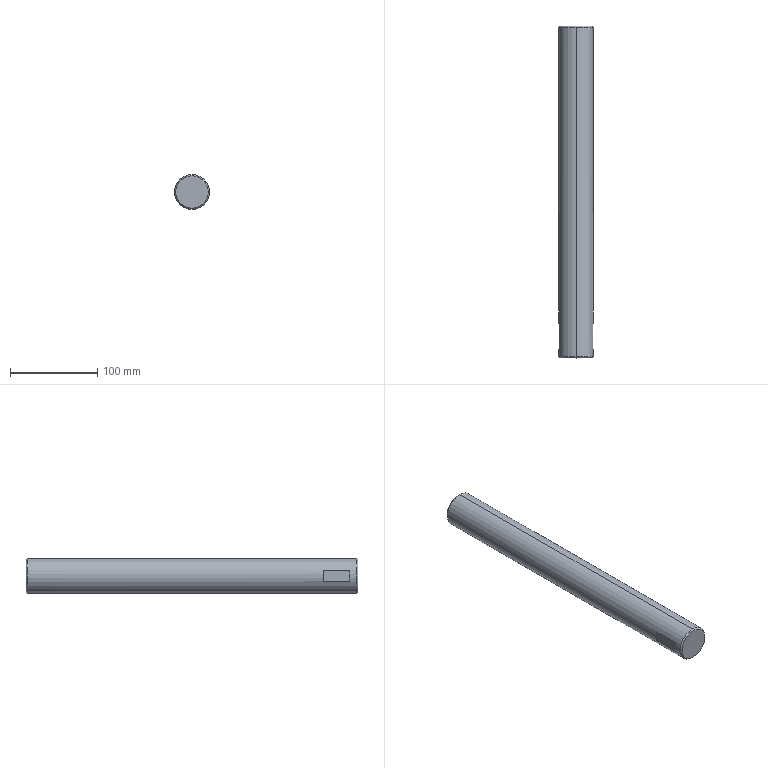Part | SolidWorks | features Chamfer 1, HoleWzd 1, ICE 1, Revolution 1 | 1 solid | 18 faces | box 40 x 380 x 40 mm | volume 474700 mm3 | plane 8 | cone 6 | cylinder 4 | commonest cylinder face diameters 10.2 x2 40 x2
STEP:
#1=CARTESIAN_POINT('',(-88.746,301.337,-5.1));
#2=VERTEX_POINT('',#1);
#3=CARTESIAN_POINT('',(-88.746,301.337,5.1));
#4=VERTEX_POINT('',#3);
#5=CARTESIAN_POINT('',(-88.746,301.337,0.));
#6=DIRECTION('',(0.,1.,0.));
#7=DIRECTION('',(0.,0.,1.));
#8=AXIS2_PLACEMENT_3D('',#5,#6,#7);
#9=CIRCLE('',#8,5.1);
#10=EDGE_CURVE('',#2,#4,#9,.T.);
#11=ORIENTED_EDGE('',*,*,#10,.F.);
#12=CARTESIAN_POINT('',(-88.746,325.337,-5.1));
#13=VERTEX_POINT('',#12);
#14=CARTESIAN_POINT('',(-88.746,325.337,-5.1));
#15=DIRECTION('',(0.,1.,0.));
#16=VECTOR('',#15,1000.);
#17=LINE('',#14,#16);
#18=EDGE_CURVE('',#2,#13,#17,.T.);
#19=ORIENTED_EDGE('',*,*,#18,.T.);
#20=CARTESIAN_POINT('',(-88.746,325.337,5.1));
#21=VERTEX_POINT('',#20);
#22=CARTESIAN_POINT('',(-88.746,325.337,0.));
#23=DIRECTION('',(0.,1.,0.));
#24=DIRECTION('',(0.,0.,1.));
#25=AXIS2_PLACEMENT_3D('',#22,#23,#24);
#26=CIRCLE('',#25,5.1);
#27=EDGE_CURVE('',#13,#21,#26,.T.);
#28=ORIENTED_EDGE('',*,*,#27,.T.);
#29=CARTESIAN_POINT('',(-88.746,325.337,5.1));
#30=DIRECTION('',(0.,1.,0.));
#31=VECTOR('',#30,1000.);
#32=LINE('',#29,#31);
#33=EDGE_CURVE('',#4,#21,#32,.T.);
#34=ORIENTED_EDGE('',*,*,#33,.F.);
#35=EDGE_LOOP('',(#11,#19,#28,#34));
#36=FACE_OUTER_BOUND('',#35,.T.);
#37=CARTESIAN_POINT('',(-88.746,325.337,0.));
#38=DIRECTION('',(0.,1.,0.));
#39=DIRECTION('',(0.,0.,1.));
#40=AXIS2_PLACEMENT_3D('',#37,#38,#39);
#41=CYLINDRICAL_SURFACE('',#40,5.1);
#42=ADVANCED_FACE('',(#36),#41,.F.);
#43=CARTESIAN_POINT('',(-88.746,298.273,0.));
#44=VERTEX_POINT('',#43);
#45=CARTESIAN_POINT('',(-88.746,301.337,5.1));
#46=DIRECTION('',(0.,0.515,0.8572));
#47=VECTOR('',#46,1000.);
#48=LINE('',#45,#47);
#49=EDGE_CURVE('',#44,#4,#48,.T.);
#50=ORIENTED_EDGE('',*,*,#49,.F.);
#51=CARTESIAN_POINT('',(-88.746,301.337,-5.1));
#52=DIRECTION('',(0.,0.515,-0.8572));
#53=VECTOR('',#52,1000.);
#54=LINE('',#51,#53);
#55=EDGE_CURVE('',#44,#2,#54,.T.);
#56=ORIENTED_EDGE('',*,*,#55,.T.);
#57=ORIENTED_EDGE('',*,*,#10,.T.);
#58=EDGE_LOOP('',(#50,#56,#57));
#59=FACE_OUTER_BOUND('',#58,.T.);
#60=CARTESIAN_POINT('',(-88.746,301.337,0.));
#61=DIRECTION('',(0.,1.,0.));
#62=DIRECTION('',(0.,0.,1.));
#63=AXIS2_PLACEMENT_3D('',#60,#61,#62);
#64=CONICAL_SURFACE('',#63,5.1,1.03);
#65=ADVANCED_FACE('',(#59),#64,.F.);
#66=CARTESIAN_POINT('',(-88.746,-54.663,-18.5));
#67=VERTEX_POINT('',#66);
#68=CARTESIAN_POINT('',(-88.746,-54.663,18.5));
#69=VERTEX_POINT('',#68);
#70=CARTESIAN_POINT('',(-88.746,-54.663,0.));
#71=DIRECTION('',(0.,-1.,0.));
#72=DIRECTION('',(0.,0.,-1.));
#73=AXIS2_PLACEMENT_3D('',#70,#71,#72);
#74=CIRCLE('',#73,18.5);
#75=EDGE_CURVE('',#67,#69,#74,.T.);
#76=ORIENTED_EDGE('',*,*,#75,.F.);
#77=CARTESIAN_POINT('',(-88.746,-53.163,-20.));
#78=VERTEX_POINT('',#77);
#79=CARTESIAN_POINT('',(-88.746,-53.163,-20.));
#80=DIRECTION('',(0.,0.7071,-0.7071));
#81=VECTOR('',#80,1000.);
#82=LINE('',#79,#81);
#83=EDGE_CURVE('',#67,#78,#82,.T.);
#84=ORIENTED_EDGE('',*,*,#83,.T.);
#85=CARTESIAN_POINT('',(-88.746,-53.163,20.));
#86=VERTEX_POINT('',#85);
#87=CARTESIAN_POINT('',(-88.746,-53.163,0.));
#88=DIRECTION('',(0.,1.,0.));
#89=DIRECTION('',(0.,0.,-1.));
#90=AXIS2_PLACEMENT_3D('',#87,#88,#89);
#91=CIRCLE('',#90,20.);
#92=EDGE_CURVE('',#86,#78,#91,.T.);
#93=ORIENTED_EDGE('',*,*,#92,.F.);
#94=CARTESIAN_POINT('',(-88.746,-53.163,20.));
#95=DIRECTION('',(0.,0.7071,0.7071));
#96=VECTOR('',#95,1000.);
#97=LINE('',#94,#96);
#98=EDGE_CURVE('',#69,#86,#97,.T.);
#99=ORIENTED_EDGE('',*,*,#98,.F.);
#100=EDGE_LOOP('',(#76,#84,#93,#99));
#101=FACE_OUTER_BOUND('',#100,.T.);
#102=CARTESIAN_POINT('',(-88.746,-53.163,0.));
#103=DIRECTION('',(0.,1.,0.));
#104=DIRECTION('',(0.,0.,1.));
#105=AXIS2_PLACEMENT_3D('',#102,#103,#104);
#106=CONICAL_SURFACE('',#105,20.,0.7854);
#107=ADVANCED_FACE('',(#101),#106,.T.);
#108=CARTESIAN_POINT('',(-88.746,325.337,18.5));
#109=VERTEX_POINT('',#108);
#110=CARTESIAN_POINT('',(-88.746,325.337,-18.5));
#111=VERTEX_POINT('',#110);
#112=CARTESIAN_POINT('',(-88.746,325.337,0.));
#113=DIRECTION('',(0.,1.,0.));
#114=DIRECTION('',(0.,0.,1.));
#115=AXIS2_PLACEMENT_3D('',#112,#113,#114);
#116=CIRCLE('',#115,18.5);
#117=EDGE_CURVE('',#109,#111,#116,.T.);
#118=ORIENTED_EDGE('',*,*,#117,.F.);
#119=CARTESIAN_POINT('',(-88.746,323.837,20.));
#120=VERTEX_POINT('',#119);
#121=CARTESIAN_POINT('',(-88.746,325.337,18.5));
#122=DIRECTION('',(0.,-0.7071,0.7071));
#123=VECTOR('',#122,1000.);
#124=LINE('',#121,#123);
#125=EDGE_CURVE('',#109,#120,#124,.T.);
#126=ORIENTED_EDGE('',*,*,#125,.T.);
#127=CARTESIAN_POINT('',(-88.746,323.837,-20.));
#128=VERTEX_POINT('',#127);
#129=CARTESIAN_POINT('',(-88.746,323.837,0.));
#130=DIRECTION('',(0.,-1.,0.));
#131=DIRECTION('',(0.,0.,1.));
#132=AXIS2_PLACEMENT_3D('',#129,#130,#131);
#133=CIRCLE('',#132,20.);
#134=EDGE_CURVE('',#128,#120,#133,.T.);
#135=ORIENTED_EDGE('',*,*,#134,.F.);
#136=CARTESIAN_POINT('',(-88.746,325.337,-18.5));
#137=DIRECTION('',(0.,-0.7071,-0.7071));
#138=VECTOR('',#137,1000.);
#139=LINE('',#136,#138);
#140=EDGE_CURVE('',#111,#128,#139,.T.);
#141=ORIENTED_EDGE('',*,*,#140,.F.);
#142=EDGE_LOOP('',(#118,#126,#135,#141));
#143=FACE_OUTER_BOUND('',#142,.T.);
#144=CARTESIAN_POINT('',(-88.746,325.337,0.));
#145=DIRECTION('',(0.,-1.,0.));
#146=DIRECTION('',(0.,0.,-1.));
#147=AXIS2_PLACEMENT_3D('',#144,#145,#146);
#148=CONICAL_SURFACE('',#147,18.5,0.7854);
#149=ADVANCED_FACE('',(#143),#148,.T.);
#150=CARTESIAN_POINT('',(-69.746,-14.663,6.245));
#151=VERTEX_POINT('',#150);
#152=CARTESIAN_POINT('',(-69.746,-44.663,6.245));
#153=VERTEX_POINT('',#152);
#154=CARTESIAN_POINT('',(-69.746,325.337,6.245));
#155=DIRECTION('',(0.,-1.,0.));
#156=VECTOR('',#155,1000.);
#157=LINE('',#154,#156);
#158=EDGE_CURVE('',#151,#153,#157,.T.);
#159=ORIENTED_EDGE('',*,*,#158,.F.);
#160=CARTESIAN_POINT('',(-69.746,-14.663,-6.245));
#161=VERTEX_POINT('',#160);
#162=CARTESIAN_POINT('',(-88.746,-14.663,0.));
#163=DIRECTION('',(0.,-1.,0.));
#164=DIRECTION('',(-1.,0.,0.));
#165=AXIS2_PLACEMENT_3D('',#162,#163,#164);
#166=CIRCLE('',#165,20.);
#167=EDGE_CURVE('',#161,#151,#166,.T.);
#168=ORIENTED_EDGE('',*,*,#167,.F.);
#169=CARTESIAN_POINT('',(-69.746,-44.663,-6.245));
#170=VERTEX_POINT('',#169);
#171=CARTESIAN_POINT('',(-69.746,325.337,-6.245));
#172=DIRECTION('',(0.,1.,0.));
#173=VECTOR('',#172,1000.);
#174=LINE('',#171,#173);
#175=EDGE_CURVE('',#170,#161,#174,.T.);
#176=ORIENTED_EDGE('',*,*,#175,.F.);
#177=CARTESIAN_POINT('',(-88.746,-44.663,0.));
#178=DIRECTION('',(0.,1.,0.));
#179=DIRECTION('',(0.,0.,-1.));
#180=AXIS2_PLACEMENT_3D('',#177,#178,#179);
#181=CIRCLE('',#180,20.);
#182=EDGE_CURVE('',#153,#170,#181,.T.);
#183=ORIENTED_EDGE('',*,*,#182,.F.);
#184=EDGE_LOOP('',(#159,#168,#176,#183));
#185=FACE_BOUND('',#184,.T.);
#186=ORIENTED_EDGE('',*,*,#92,.T.);
#187=CARTESIAN_POINT('',(-88.746,325.337,-20.));
#188=DIRECTION('',(0.,1.,0.));
#189=VECTOR('',#188,1000.);
#190=LINE('',#187,#189);
#191=EDGE_CURVE('',#78,#128,#190,.T.);
#192=ORIENTED_EDGE('',*,*,#191,.T.);
#193=ORIENTED_EDGE('',*,*,#134,.T.);
#194=CARTESIAN_POINT('',(-88.746,325.337,20.));
#195=DIRECTION('',(0.,1.,0.));
#196=VECTOR('',#195,1000.);
#197=LINE('',#194,#196);
#198=EDGE_CURVE('',#86,#120,#197,.T.);
#199=ORIENTED_EDGE('',*,*,#198,.F.);
#200=EDGE_LOOP('',(#186,#192,#193,#199));
#201=FACE_OUTER_BOUND('',#200,.T.);
#202=CARTESIAN_POINT('',(-88.746,325.337,0.));
#203=DIRECTION('',(0.,1.,0.));
#204=DIRECTION('',(0.,0.,1.));
#205=AXIS2_PLACEMENT_3D('',#202,#203,#204);
#206=CYLINDRICAL_SURFACE('',#205,20.);
#207=ADVANCED_FACE('',(#185,#201),#206,.T.);
#208=CARTESIAN_POINT('',(-88.746,325.337,0.));
#209=DIRECTION('',(0.,1.,0.));
#210=DIRECTION('',(0.,0.,1.));
#211=AXIS2_PLACEMENT_3D('',#208,#209,#210);
#212=CIRCLE('',#211,5.1);
#213=EDGE_CURVE('',#21,#13,#212,.T.);
#214=ORIENTED_EDGE('',*,*,#213,.F.);
#215=ORIENTED_EDGE('',*,*,#27,.F.);
#216=EDGE_LOOP('',(#214,#215));
#217=FACE_BOUND('',#216,.T.);
#218=CARTESIAN_POINT('',(-88.746,325.337,0.));
#219=DIRECTION('',(0.,1.,0.));
#220=DIRECTION('',(0.,0.,1.));
#221=AXIS2_PLACEMENT_3D('',#218,#219,#220);
#222=CIRCLE('',#221,18.5);
#223=EDGE_CURVE('',#111,#109,#222,.T.);
#224=ORIENTED_EDGE('',*,*,#223,.T.);
#225=ORIENTED_EDGE('',*,*,#117,.T.);
#226=EDGE_LOOP('',(#224,#225));
#227=FACE_OUTER_BOUND('',#226,.T.);
#228=CARTESIAN_POINT('',(-108.746,325.337,0.));
#229=DIRECTION('',(0.,1.,0.));
#230=DIRECTION('',(0.,0.,1.));
#231=AXIS2_PLACEMENT_3D('',#228,#229,#230);
#232=PLANE('',#231);
#233=ADVANCED_FACE('',(#217,#227),#232,.T.);
#234=ORIENTED_EDGE('',*,*,#191,.F.);
#235=CARTESIAN_POINT('',(-88.746,-53.163,0.));
#236=DIRECTION('',(0.,1.,0.));
#237=DIRECTION('',(0.,0.,-1.));
#238=AXIS2_PLACEMENT_3D('',#235,#236,#237);
#239=CIRCLE('',#238,20.);
#240=EDGE_CURVE('',#78,#86,#239,.T.);
#241=ORIENTED_EDGE('',*,*,#240,.T.);
#242=ORIENTED_EDGE('',*,*,#198,.T.);
#243=CARTESIAN_POINT('',(-88.746,323.837,0.));
#244=DIRECTION('',(0.,-1.,0.));
#245=DIRECTION('',(0.,0.,1.));
#246=AXIS2_PLACEMENT_3D('',#243,#244,#245);
#247=CIRCLE('',#246,20.);
#248=EDGE_CURVE('',#120,#128,#247,.T.);
#249=ORIENTED_EDGE('',*,*,#248,.T.);
#250=EDGE_LOOP('',(#234,#241,#242,#249));
#251=FACE_OUTER_BOUND('',#250,.T.);
#252=CARTESIAN_POINT('',(-107.746,-14.663,-6.245));
#253=VERTEX_POINT('',#252);
#254=CARTESIAN_POINT('',(-107.746,-44.663,-6.245));
#255=VERTEX_POINT('',#254);
#256=CARTESIAN_POINT('',(-107.746,325.337,-6.245));
#257=DIRECTION('',(0.,-1.,0.));
#258=VECTOR('',#257,1000.);
#259=LINE('',#256,#258);
#260=EDGE_CURVE('',#253,#255,#259,.T.);
#261=ORIENTED_EDGE('',*,*,#260,.F.);
#262=CARTESIAN_POINT('',(-107.746,-14.663,6.245));
#263=VERTEX_POINT('',#262);
#264=CARTESIAN_POINT('',(-88.746,-14.663,0.));
#265=DIRECTION('',(0.,-1.,0.));
#266=DIRECTION('',(-1.,0.,0.));
#267=AXIS2_PLACEMENT_3D('',#264,#265,#266);
#268=CIRCLE('',#267,20.);
#269=EDGE_CURVE('',#263,#253,#268,.T.);
#270=ORIENTED_EDGE('',*,*,#269,.F.);
#271=CARTESIAN_POINT('',(-107.746,-44.663,6.245));
#272=VERTEX_POINT('',#271);
#273=CARTESIAN_POINT('',(-107.746,325.337,6.245));
#274=DIRECTION('',(0.,1.,0.));
#275=VECTOR('',#274,1000.);
#276=LINE('',#273,#275);
#277=EDGE_CURVE('',#272,#263,#276,.T.);
#278=ORIENTED_EDGE('',*,*,#277,.F.);
#279=CARTESIAN_POINT('',(-88.746,-44.663,0.));
#280=DIRECTION('',(0.,1.,0.));
#281=DIRECTION('',(0.,0.,-1.));
#282=AXIS2_PLACEMENT_3D('',#279,#280,#281);
#283=CIRCLE('',#282,20.);
#284=EDGE_CURVE('',#255,#272,#283,.T.);
#285=ORIENTED_EDGE('',*,*,#284,.F.);
#286=EDGE_LOOP('',(#261,#270,#278,#285));
#287=FACE_BOUND('',#286,.T.);
#288=CARTESIAN_POINT('',(-88.746,325.337,0.));
#289=DIRECTION('',(0.,1.,0.));
#290=DIRECTION('',(0.,0.,1.));
#291=AXIS2_PLACEMENT_3D('',#288,#289,#290);
#292=CYLINDRICAL_SURFACE('',#291,20.);
#293=ADVANCED_FACE('',(#251,#287),#292,.T.);
#294=CARTESIAN_POINT('',(-88.746,-54.663,0.));
#295=DIRECTION('',(0.,-1.,0.));
#296=DIRECTION('',(0.,0.,-1.));
#297=AXIS2_PLACEMENT_3D('',#294,#295,#296);
#298=CIRCLE('',#297,18.5);
#299=EDGE_CURVE('',#69,#67,#298,.T.);
#300=ORIENTED_EDGE('',*,*,#299,.T.);
#301=ORIENTED_EDGE('',*,*,#75,.T.);
#302=EDGE_LOOP('',(#300,#301));
#303=FACE_OUTER_BOUND('',#302,.T.);
#304=CARTESIAN_POINT('',(-108.746,-54.663,0.));
#305=DIRECTION('',(0.,-1.,0.));
#306=DIRECTION('',(0.,0.,-1.));
#307=AXIS2_PLACEMENT_3D('',#304,#305,#306);
#308=PLANE('',#307);
#309=ADVANCED_FACE('',(#303),#308,.T.);
#310=ORIENTED_EDGE('',*,*,#167,.T.);
#311=CARTESIAN_POINT('',(-69.746,-14.663,-20.));
#312=DIRECTION('',(0.,0.,1.));
#313=VECTOR('',#312,1000.);
#314=LINE('',#311,#313);
#315=EDGE_CURVE('',#161,#151,#314,.T.);
#316=ORIENTED_EDGE('',*,*,#315,.F.);
#317=EDGE_LOOP('',(#310,#316));
#318=FACE_OUTER_BOUND('',#317,.T.);
#319=CARTESIAN_POINT('',(-68.746,-14.663,-20.));
#320=DIRECTION('',(0.,1.,0.));
#321=DIRECTION('',(-1.,0.,0.));
#322=AXIS2_PLACEMENT_3D('',#319,#320,#321);
#323=PLANE('',#322);
#324=ADVANCED_FACE('',(#318),#323,.F.);
#325=CARTESIAN_POINT('',(-69.746,-44.663,-20.));
#326=DIRECTION('',(0.,0.,1.));
#327=VECTOR('',#326,1000.);
#328=LINE('',#325,#327);
#329=EDGE_CURVE('',#170,#153,#328,.T.);
#330=ORIENTED_EDGE('',*,*,#329,.T.);
#331=ORIENTED_EDGE('',*,*,#182,.T.);
#332=EDGE_LOOP('',(#330,#331));
#333=FACE_OUTER_BOUND('',#332,.T.);
#334=CARTESIAN_POINT('',(-68.746,-44.663,-20.));
#335=DIRECTION('',(0.,-1.,0.));
#336=DIRECTION('',(0.,0.,-1.));
#337=AXIS2_PLACEMENT_3D('',#334,#335,#336);
#338=PLANE('',#337);
#339=ADVANCED_FACE('',(#333),#338,.F.);
#340=ORIENTED_EDGE('',*,*,#158,.T.);
#341=ORIENTED_EDGE('',*,*,#329,.F.);
#342=ORIENTED_EDGE('',*,*,#175,.T.);
#343=ORIENTED_EDGE('',*,*,#315,.T.);
#344=EDGE_LOOP('',(#340,#341,#342,#343));
#345=FACE_OUTER_BOUND('',#344,.T.);
#346=CARTESIAN_POINT('',(-69.746,-14.663,-20.));
#347=DIRECTION('',(-1.,0.,0.));
#348=DIRECTION('',(0.,0.,1.));
#349=AXIS2_PLACEMENT_3D('',#346,#347,#348);
#350=PLANE('',#349);
#351=ADVANCED_FACE('',(#345),#350,.F.);
#352=ORIENTED_EDGE('',*,*,#269,.T.);
#353=CARTESIAN_POINT('',(-107.746,-14.663,-20.));
#354=DIRECTION('',(0.,0.,1.));
#355=VECTOR('',#354,1000.);
#356=LINE('',#353,#355);
#357=EDGE_CURVE('',#253,#263,#356,.T.);
#358=ORIENTED_EDGE('',*,*,#357,.T.);
#359=EDGE_LOOP('',(#352,#358));
#360=FACE_OUTER_BOUND('',#359,.T.);
#361=CARTESIAN_POINT('',(-108.746,-14.663,-20.));
#362=DIRECTION('',(0.,1.,0.));
#363=DIRECTION('',(-1.,0.,0.));
#364=AXIS2_PLACEMENT_3D('',#361,#362,#363);
#365=PLANE('',#364);
#366=ADVANCED_FACE('',(#360),#365,.F.);
#367=ORIENTED_EDGE('',*,*,#260,.T.);
#368=CARTESIAN_POINT('',(-107.746,-44.663,-20.));
#369=DIRECTION('',(0.,0.,1.));
#370=VECTOR('',#369,1000.);
#371=LINE('',#368,#370);
#372=EDGE_CURVE('',#255,#272,#371,.T.);
#373=ORIENTED_EDGE('',*,*,#372,.T.);
#374=ORIENTED_EDGE('',*,*,#277,.T.);
#375=ORIENTED_EDGE('',*,*,#357,.F.);
#376=EDGE_LOOP('',(#367,#373,#374,#375));
#377=FACE_OUTER_BOUND('',#376,.T.);
#378=CARTESIAN_POINT('',(-107.746,-14.663,-20.));
#379=DIRECTION('',(1.,0.,0.));
#380=DIRECTION('',(0.,0.,-1.));
#381=AXIS2_PLACEMENT_3D('',#378,#379,#380);
#382=PLANE('',#381);
#383=ADVANCED_FACE('',(#377),#382,.F.);
#384=ORIENTED_EDGE('',*,*,#372,.F.);
#385=ORIENTED_EDGE('',*,*,#284,.T.);
#386=EDGE_LOOP('',(#384,#385));
#387=FACE_OUTER_BOUND('',#386,.T.);
#388=CARTESIAN_POINT('',(-108.746,-44.663,-20.));
#389=DIRECTION('',(0.,-1.,0.));
#390=DIRECTION('',(0.,0.,-1.));
#391=AXIS2_PLACEMENT_3D('',#388,#389,#390);
#392=PLANE('',#391);
#393=ADVANCED_FACE('',(#387),#392,.F.);
#394=ORIENTED_EDGE('',*,*,#125,.F.);
#395=ORIENTED_EDGE('',*,*,#223,.F.);
#396=ORIENTED_EDGE('',*,*,#140,.T.);
#397=ORIENTED_EDGE('',*,*,#248,.F.);
#398=EDGE_LOOP('',(#394,#395,#396,#397));
#399=FACE_OUTER_BOUND('',#398,.T.);
#400=CARTESIAN_POINT('',(-88.746,325.337,0.));
#401=DIRECTION('',(0.,-1.,0.));
#402=DIRECTION('',(0.,0.,-1.));
#403=AXIS2_PLACEMENT_3D('',#400,#401,#402);
#404=CONICAL_SURFACE('',#403,18.5,0.7854);
#405=ADVANCED_FACE('',(#399),#404,.T.);
#406=ORIENTED_EDGE('',*,*,#83,.F.);
#407=ORIENTED_EDGE('',*,*,#299,.F.);
#408=ORIENTED_EDGE('',*,*,#98,.T.);
#409=ORIENTED_EDGE('',*,*,#240,.F.);
#410=EDGE_LOOP('',(#406,#407,#408,#409));
#411=FACE_OUTER_BOUND('',#410,.T.);
#412=CARTESIAN_POINT('',(-88.746,-53.163,0.));
#413=DIRECTION('',(0.,1.,0.));
#414=DIRECTION('',(0.,0.,1.));
#415=AXIS2_PLACEMENT_3D('',#412,#413,#414);
#416=CONICAL_SURFACE('',#415,20.,0.7854);
#417=ADVANCED_FACE('',(#411),#416,.T.);
#418=ORIENTED_EDGE('',*,*,#55,.F.);
#419=ORIENTED_EDGE('',*,*,#49,.T.);
#420=CARTESIAN_POINT('',(-88.746,301.337,0.));
#421=DIRECTION('',(0.,1.,0.));
#422=DIRECTION('',(0.,0.,1.));
#423=AXIS2_PLACEMENT_3D('',#420,#421,#422);
#424=CIRCLE('',#423,5.1);
#425=EDGE_CURVE('',#4,#2,#424,.T.);
#426=ORIENTED_EDGE('',*,*,#425,.T.);
#427=EDGE_LOOP('',(#418,#419,#426));
#428=FACE_OUTER_BOUND('',#427,.T.);
#429=CARTESIAN_POINT('',(-88.746,301.337,0.));
#430=DIRECTION('',(0.,1.,0.));
#431=DIRECTION('',(0.,0.,1.));
#432=AXIS2_PLACEMENT_3D('',#429,#430,#431);
#433=CONICAL_SURFACE('',#432,5.1,1.03);
#434=ADVANCED_FACE('',(#428),#433,.F.);
#435=ORIENTED_EDGE('',*,*,#18,.F.);
#436=ORIENTED_EDGE('',*,*,#425,.F.);
#437=ORIENTED_EDGE('',*,*,#33,.T.);
#438=ORIENTED_EDGE('',*,*,#213,.T.);
#439=EDGE_LOOP('',(#435,#436,#437,#438));
#440=FACE_OUTER_BOUND('',#439,.T.);
#441=CARTESIAN_POINT('',(-88.746,325.337,0.));
#442=DIRECTION('',(0.,1.,0.));
#443=DIRECTION('',(0.,0.,1.));
#444=AXIS2_PLACEMENT_3D('',#441,#442,#443);
#445=CYLINDRICAL_SURFACE('',#444,5.1);
#446=ADVANCED_FACE('',(#440),#445,.F.);
#447=CLOSED_SHELL('',(#42,#65,#107,#149,#207,#233,#293,#309,#324,#339,#351,#366,#383,#393,#405,#417,#434,#446));
#448=MANIFOLD_SOLID_BREP('',#447);
#449=CARTESIAN_POINT('',(0.,0.,0.));
#450=DIRECTION('',(0.,0.,1.));
#451=DIRECTION('',(1.,0.,0.));
#452=AXIS2_PLACEMENT_3D('',#449,#450,#451);
#453=(LENGTH_UNIT()NAMED_UNIT(*)SI_UNIT(.MILLI.,.METRE.));
#454=UNCERTAINTY_MEASURE_WITH_UNIT(LENGTH_MEASURE(0.00001),#453,'','');
#455=(NAMED_UNIT(*)PLANE_ANGLE_UNIT()SI_UNIT($,.RADIAN.));
#456=(NAMED_UNIT(*)SI_UNIT($,.STERADIAN.)SOLID_ANGLE_UNIT());
#457=(GEOMETRIC_REPRESENTATION_CONTEXT(3)GLOBAL_UNCERTAINTY_ASSIGNED_CONTEXT((#454))GLOBAL_UNIT_ASSIGNED_CONTEXT((#453,#455,#456))REPRESENTATION_CONTEXT('',''));
#458=ADVANCED_BREP_SHAPE_REPRESENTATION('',(#448,#452),#457);